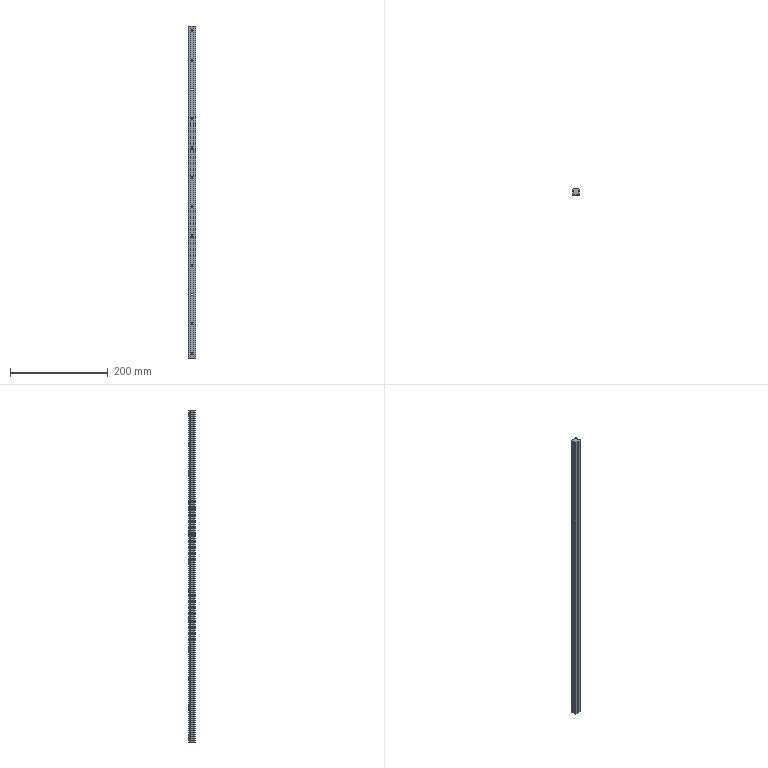Part | SolidWorks | features ICE 2, BaseBody 1, HoleWzd 1 | 1 solid | 110 faces | box 15 x 12.5 x 680 mm | volume 106806 mm3 | cylinder 66 | plane 44 | commonest cylinder face diameters 4.5 x24 8 x24 0.6 x11 3 x5 1 x2